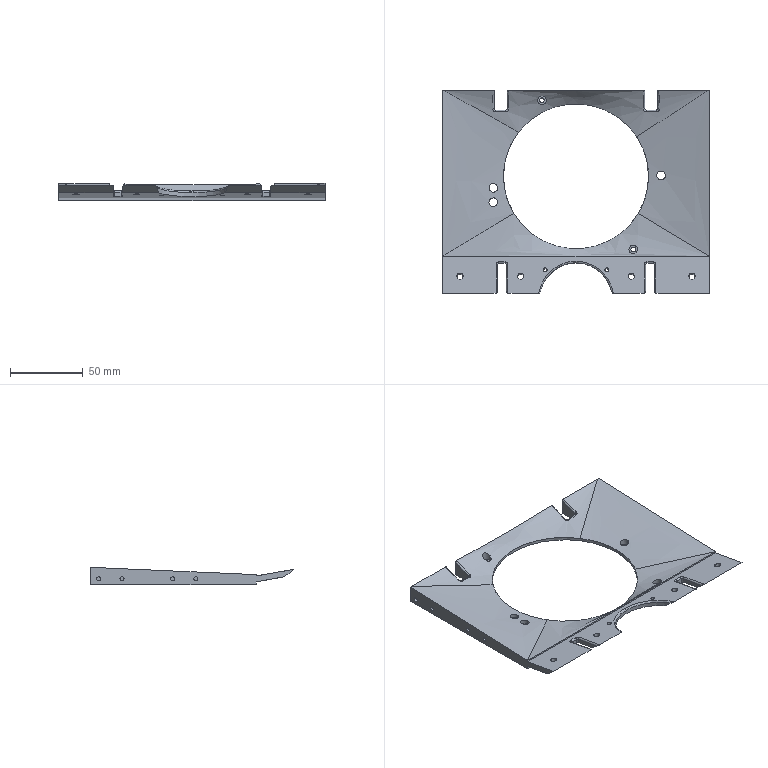Part | SolidWorks | features ICE 17, 3DProfileFeature 8, Fillet 3, Extrusion 1, MirrorPattern 1 | 1 solid | 115 faces | box 184 x 140.059 x 11.963 mm | volume 87772 mm3 | cylinder 59 | plane 36 | spline 20 | commonest cylinder face diameters 2.8 x20 2 x14 6 x10 4.3 x8 3.2 x4 100 x2